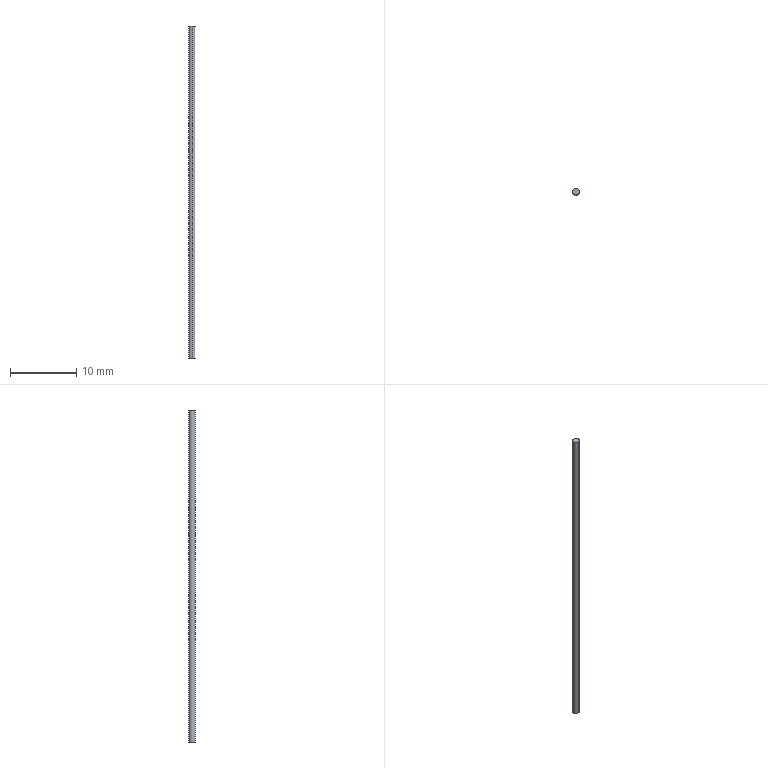Part | STEP file | LR-ZH500CP-Part-3-3 | 1 solid | 4 faces | box 1 x 1 x 50 mm | volume 39.27 mm3 | cylinder 2 | plane 2 | commonest cylinder face diameters 1 x2
STEP:
#1=CARTESIAN_POINT('',(0.,-5.4,450.));
#2=VERTEX_POINT('',#1);
#3=CARTESIAN_POINT('',(0.,-4.4,450.));
#4=VERTEX_POINT('',#3);
#5=CARTESIAN_POINT('',(0.,-4.9,450.));
#6=DIRECTION('',(0.,0.,1.));
#7=DIRECTION('',(0.,-1.,0.));
#8=AXIS2_PLACEMENT_3D('',#5,#6,#7);
#9=CIRCLE('',#8,0.5);
#10=EDGE_CURVE('',#2,#4,#9,.T.);
#11=ORIENTED_EDGE('',*,*,#10,.T.);
#12=CARTESIAN_POINT('',(0.,-4.4,500.));
#13=VERTEX_POINT('',#12);
#14=CARTESIAN_POINT('',(0.,-4.4,450.));
#15=DIRECTION('',(0.,0.,1.));
#16=VECTOR('',#15,1000.);
#17=LINE('',#14,#16);
#18=EDGE_CURVE('',#4,#13,#17,.T.);
#19=ORIENTED_EDGE('',*,*,#18,.T.);
#20=CARTESIAN_POINT('',(0.,-5.4,500.));
#21=VERTEX_POINT('',#20);
#22=CARTESIAN_POINT('',(0.,-4.9,500.));
#23=DIRECTION('',(0.,0.,-1.));
#24=DIRECTION('',(0.,1.,0.));
#25=AXIS2_PLACEMENT_3D('',#22,#23,#24);
#26=CIRCLE('',#25,0.5);
#27=EDGE_CURVE('',#13,#21,#26,.T.);
#28=ORIENTED_EDGE('',*,*,#27,.T.);
#29=CARTESIAN_POINT('',(0.,-5.4,450.));
#30=DIRECTION('',(0.,0.,1.));
#31=VECTOR('',#30,1000.);
#32=LINE('',#29,#31);
#33=EDGE_CURVE('',#2,#21,#32,.T.);
#34=ORIENTED_EDGE('',*,*,#33,.F.);
#35=EDGE_LOOP('',(#11,#19,#28,#34));
#36=FACE_OUTER_BOUND('',#35,.T.);
#37=CARTESIAN_POINT('',(0.,-4.9,450.));
#38=DIRECTION('',(0.,0.,1.));
#39=DIRECTION('',(0.,-1.,0.));
#40=AXIS2_PLACEMENT_3D('',#37,#38,#39);
#41=CYLINDRICAL_SURFACE('',#40,0.5);
#42=ADVANCED_FACE('',(#36),#41,.T.);
#43=CARTESIAN_POINT('',(0.,-4.9,500.));
#44=DIRECTION('',(0.,0.,-1.));
#45=DIRECTION('',(0.,1.,0.));
#46=AXIS2_PLACEMENT_3D('',#43,#44,#45);
#47=CIRCLE('',#46,0.5);
#48=EDGE_CURVE('',#21,#13,#47,.T.);
#49=ORIENTED_EDGE('',*,*,#48,.F.);
#50=ORIENTED_EDGE('',*,*,#27,.F.);
#51=EDGE_LOOP('',(#49,#50));
#52=FACE_OUTER_BOUND('',#51,.T.);
#53=CARTESIAN_POINT('',(0.,-4.9,500.));
#54=DIRECTION('',(0.,0.,1.));
#55=DIRECTION('',(0.,-1.,0.));
#56=AXIS2_PLACEMENT_3D('',#53,#54,#55);
#57=PLANE('',#56);
#58=ADVANCED_FACE('',(#52),#57,.T.);
#59=ORIENTED_EDGE('',*,*,#10,.F.);
#60=CARTESIAN_POINT('',(0.,-4.9,450.));
#61=DIRECTION('',(0.,0.,1.));
#62=DIRECTION('',(0.,-1.,0.));
#63=AXIS2_PLACEMENT_3D('',#60,#61,#62);
#64=CIRCLE('',#63,0.5);
#65=EDGE_CURVE('',#4,#2,#64,.T.);
#66=ORIENTED_EDGE('',*,*,#65,.F.);
#67=EDGE_LOOP('',(#59,#66));
#68=FACE_OUTER_BOUND('',#67,.T.);
#69=CARTESIAN_POINT('',(0.,-4.9,450.));
#70=DIRECTION('',(0.,0.,-1.));
#71=DIRECTION('',(0.,1.,0.));
#72=AXIS2_PLACEMENT_3D('',#69,#70,#71);
#73=PLANE('',#72);
#74=ADVANCED_FACE('',(#68),#73,.T.);
#75=ORIENTED_EDGE('',*,*,#18,.F.);
#76=ORIENTED_EDGE('',*,*,#65,.T.);
#77=ORIENTED_EDGE('',*,*,#33,.T.);
#78=ORIENTED_EDGE('',*,*,#48,.T.);
#79=EDGE_LOOP('',(#75,#76,#77,#78));
#80=FACE_OUTER_BOUND('',#79,.T.);
#81=CARTESIAN_POINT('',(0.,-4.9,450.));
#82=DIRECTION('',(0.,0.,1.));
#83=DIRECTION('',(0.,-1.,0.));
#84=AXIS2_PLACEMENT_3D('',#81,#82,#83);
#85=CYLINDRICAL_SURFACE('',#84,0.5);
#86=ADVANCED_FACE('',(#80),#85,.T.);
#87=CLOSED_SHELL('',(#42,#58,#74,#86));
#88=MANIFOLD_SOLID_BREP('',#87);
#89=CARTESIAN_POINT('',(0.,0.,0.));
#90=DIRECTION('',(0.,0.,1.));
#91=DIRECTION('',(1.,0.,0.));
#92=AXIS2_PLACEMENT_3D('',#89,#90,#91);
#93=(LENGTH_UNIT()NAMED_UNIT(*)SI_UNIT(.MILLI.,.METRE.));
#94=UNCERTAINTY_MEASURE_WITH_UNIT(LENGTH_MEASURE(0.00001),#93,'','');
#95=(NAMED_UNIT(*)PLANE_ANGLE_UNIT()SI_UNIT($,.RADIAN.));
#96=(NAMED_UNIT(*)SI_UNIT($,.STERADIAN.)SOLID_ANGLE_UNIT());
#97=(GEOMETRIC_REPRESENTATION_CONTEXT(3)GLOBAL_UNCERTAINTY_ASSIGNED_CONTEXT((#94))GLOBAL_UNIT_ASSIGNED_CONTEXT((#93,#95,#96))REPRESENTATION_CONTEXT('',''));
#98=ADVANCED_BREP_SHAPE_REPRESENTATION('',(#88,#92),#97);